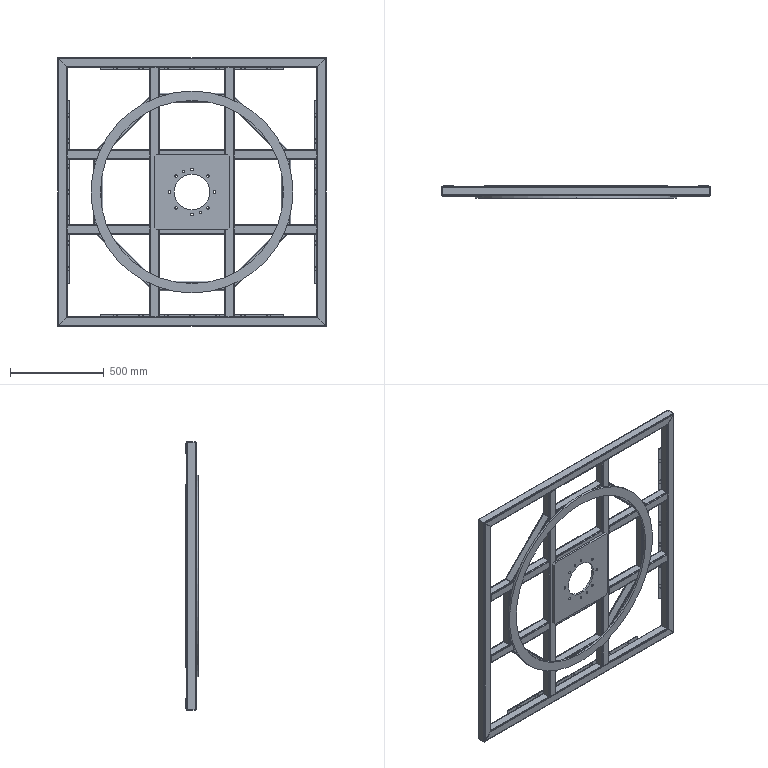Part | SolidWorks | features BaseBody 26 | 26 solids | 838 faces | box 1430 x 67 x 1430 mm | volume 10727626 mm3 | cylinder 586 | plane 252 | commonest cylinder face diameters 4.2 x368 5 x112 10 x80 13.5 x16 12 x4 190 x2